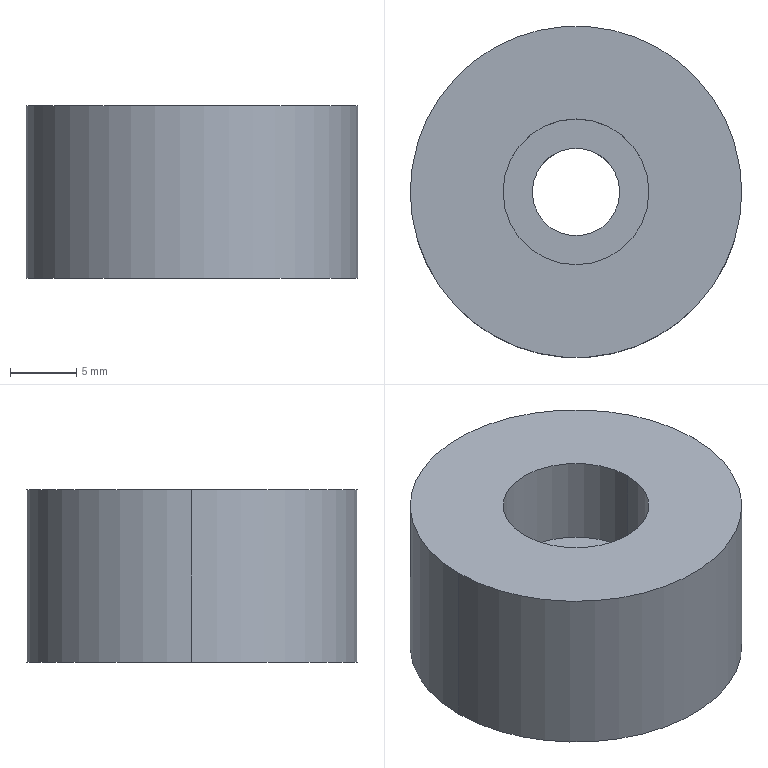Part | SolidWorks | features Extrusion 1, HoleWzd 1 | 1 solid | 9 faces | box 25 x 25 x 13 mm | volume 5523 mm3 | cylinder 6 | plane 3 | commonest cylinder face diameters 6.6 x2 11 x2 25 x2
STEP:
#1=CARTESIAN_POINT('',(-5.5,0.,6.2));
#2=VERTEX_POINT('',#1);
#3=CARTESIAN_POINT('',(5.5,0.,6.2));
#4=VERTEX_POINT('',#3);
#5=CARTESIAN_POINT('',(0.,0.,6.2));
#6=DIRECTION('',(0.,0.,1.));
#7=DIRECTION('',(1.,0.,0.));
#8=AXIS2_PLACEMENT_3D('',#5,#6,#7);
#9=CIRCLE('',#8,5.5);
#10=EDGE_CURVE('',#2,#4,#9,.T.);
#11=ORIENTED_EDGE('',*,*,#10,.F.);
#12=CARTESIAN_POINT('',(-5.5,0.,13.));
#13=VERTEX_POINT('',#12);
#14=CARTESIAN_POINT('',(-5.5,0.,13.));
#15=DIRECTION('',(0.,0.,1.));
#16=VECTOR('',#15,1000.);
#17=LINE('',#14,#16);
#18=EDGE_CURVE('',#2,#13,#17,.T.);
#19=ORIENTED_EDGE('',*,*,#18,.T.);
#20=CARTESIAN_POINT('',(5.5,0.,13.));
#21=VERTEX_POINT('',#20);
#22=CARTESIAN_POINT('',(0.,0.,13.));
#23=DIRECTION('',(0.,0.,1.));
#24=DIRECTION('',(1.,0.,0.));
#25=AXIS2_PLACEMENT_3D('',#22,#23,#24);
#26=CIRCLE('',#25,5.5);
#27=EDGE_CURVE('',#13,#21,#26,.T.);
#28=ORIENTED_EDGE('',*,*,#27,.T.);
#29=CARTESIAN_POINT('',(5.5,0.,13.));
#30=DIRECTION('',(0.,0.,1.));
#31=VECTOR('',#30,1000.);
#32=LINE('',#29,#31);
#33=EDGE_CURVE('',#4,#21,#32,.T.);
#34=ORIENTED_EDGE('',*,*,#33,.F.);
#35=EDGE_LOOP('',(#11,#19,#28,#34));
#36=FACE_OUTER_BOUND('',#35,.T.);
#37=CARTESIAN_POINT('',(0.,0.,13.));
#38=DIRECTION('',(0.,0.,1.));
#39=DIRECTION('',(1.,0.,0.));
#40=AXIS2_PLACEMENT_3D('',#37,#38,#39);
#41=CYLINDRICAL_SURFACE('',#40,5.5);
#42=ADVANCED_FACE('',(#36),#41,.F.);
#43=CARTESIAN_POINT('',(-3.3,0.,0.));
#44=VERTEX_POINT('',#43);
#45=CARTESIAN_POINT('',(3.3,0.,0.));
#46=VERTEX_POINT('',#45);
#47=CARTESIAN_POINT('',(0.,0.,0.));
#48=DIRECTION('',(0.,0.,1.));
#49=DIRECTION('',(1.,0.,0.));
#50=AXIS2_PLACEMENT_3D('',#47,#48,#49);
#51=CIRCLE('',#50,3.3);
#52=EDGE_CURVE('',#44,#46,#51,.T.);
#53=ORIENTED_EDGE('',*,*,#52,.F.);
#54=CARTESIAN_POINT('',(-3.3,0.,6.2));
#55=VERTEX_POINT('',#54);
#56=CARTESIAN_POINT('',(-3.3,0.,13.));
#57=DIRECTION('',(0.,0.,1.));
#58=VECTOR('',#57,1000.);
#59=LINE('',#56,#58);
#60=EDGE_CURVE('',#44,#55,#59,.T.);
#61=ORIENTED_EDGE('',*,*,#60,.T.);
#62=CARTESIAN_POINT('',(3.3,0.,6.2));
#63=VERTEX_POINT('',#62);
#64=CARTESIAN_POINT('',(0.,0.,6.2));
#65=DIRECTION('',(0.,0.,1.));
#66=DIRECTION('',(1.,0.,0.));
#67=AXIS2_PLACEMENT_3D('',#64,#65,#66);
#68=CIRCLE('',#67,3.3);
#69=EDGE_CURVE('',#55,#63,#68,.T.);
#70=ORIENTED_EDGE('',*,*,#69,.T.);
#71=CARTESIAN_POINT('',(3.3,0.,13.));
#72=DIRECTION('',(0.,0.,1.));
#73=VECTOR('',#72,1000.);
#74=LINE('',#71,#73);
#75=EDGE_CURVE('',#46,#63,#74,.T.);
#76=ORIENTED_EDGE('',*,*,#75,.F.);
#77=EDGE_LOOP('',(#53,#61,#70,#76));
#78=FACE_OUTER_BOUND('',#77,.T.);
#79=CARTESIAN_POINT('',(0.,0.,13.));
#80=DIRECTION('',(0.,0.,1.));
#81=DIRECTION('',(1.,0.,0.));
#82=AXIS2_PLACEMENT_3D('',#79,#80,#81);
#83=CYLINDRICAL_SURFACE('',#82,3.3);
#84=ADVANCED_FACE('',(#78),#83,.F.);
#85=CARTESIAN_POINT('',(12.5,0.,13.));
#86=VERTEX_POINT('',#85);
#87=CARTESIAN_POINT('',(-12.5,0.,13.));
#88=VERTEX_POINT('',#87);
#89=CARTESIAN_POINT('',(0.,0.,13.));
#90=DIRECTION('',(0.,0.,1.));
#91=DIRECTION('',(1.,0.,0.));
#92=AXIS2_PLACEMENT_3D('',#89,#90,#91);
#93=CIRCLE('',#92,12.5);
#94=EDGE_CURVE('',#86,#88,#93,.T.);
#95=ORIENTED_EDGE('',*,*,#94,.F.);
#96=CARTESIAN_POINT('',(12.5,0.,0.));
#97=VERTEX_POINT('',#96);
#98=CARTESIAN_POINT('',(12.5,0.,13.));
#99=DIRECTION('',(0.,0.,-1.));
#100=VECTOR('',#99,1000.);
#101=LINE('',#98,#100);
#102=EDGE_CURVE('',#86,#97,#101,.T.);
#103=ORIENTED_EDGE('',*,*,#102,.T.);
#104=CARTESIAN_POINT('',(-12.5,0.,0.));
#105=VERTEX_POINT('',#104);
#106=CARTESIAN_POINT('',(0.,0.,0.));
#107=DIRECTION('',(0.,0.,1.));
#108=DIRECTION('',(1.,0.,0.));
#109=AXIS2_PLACEMENT_3D('',#106,#107,#108);
#110=CIRCLE('',#109,12.5);
#111=EDGE_CURVE('',#97,#105,#110,.T.);
#112=ORIENTED_EDGE('',*,*,#111,.T.);
#113=CARTESIAN_POINT('',(-12.5,0.,13.));
#114=DIRECTION('',(0.,0.,-1.));
#115=VECTOR('',#114,1000.);
#116=LINE('',#113,#115);
#117=EDGE_CURVE('',#88,#105,#116,.T.);
#118=ORIENTED_EDGE('',*,*,#117,.F.);
#119=EDGE_LOOP('',(#95,#103,#112,#118));
#120=FACE_OUTER_BOUND('',#119,.T.);
#121=CARTESIAN_POINT('',(0.,0.,13.));
#122=DIRECTION('',(0.,0.,-1.));
#123=DIRECTION('',(-1.,0.,0.));
#124=AXIS2_PLACEMENT_3D('',#121,#122,#123);
#125=CYLINDRICAL_SURFACE('',#124,12.5);
#126=ADVANCED_FACE('',(#120),#125,.T.);
#127=ORIENTED_EDGE('',*,*,#102,.F.);
#128=CARTESIAN_POINT('',(0.,0.,13.));
#129=DIRECTION('',(0.,0.,1.));
#130=DIRECTION('',(1.,0.,0.));
#131=AXIS2_PLACEMENT_3D('',#128,#129,#130);
#132=CIRCLE('',#131,12.5);
#133=EDGE_CURVE('',#88,#86,#132,.T.);
#134=ORIENTED_EDGE('',*,*,#133,.F.);
#135=ORIENTED_EDGE('',*,*,#117,.T.);
#136=CARTESIAN_POINT('',(0.,0.,0.));
#137=DIRECTION('',(0.,0.,1.));
#138=DIRECTION('',(1.,0.,0.));
#139=AXIS2_PLACEMENT_3D('',#136,#137,#138);
#140=CIRCLE('',#139,12.5);
#141=EDGE_CURVE('',#105,#97,#140,.T.);
#142=ORIENTED_EDGE('',*,*,#141,.T.);
#143=EDGE_LOOP('',(#127,#134,#135,#142));
#144=FACE_OUTER_BOUND('',#143,.T.);
#145=CARTESIAN_POINT('',(0.,0.,13.));
#146=DIRECTION('',(0.,0.,-1.));
#147=DIRECTION('',(-1.,0.,0.));
#148=AXIS2_PLACEMENT_3D('',#145,#146,#147);
#149=CYLINDRICAL_SURFACE('',#148,12.5);
#150=ADVANCED_FACE('',(#144),#149,.T.);
#151=CARTESIAN_POINT('',(0.,0.,13.));
#152=DIRECTION('',(0.,0.,1.));
#153=DIRECTION('',(1.,0.,0.));
#154=AXIS2_PLACEMENT_3D('',#151,#152,#153);
#155=CIRCLE('',#154,5.5);
#156=EDGE_CURVE('',#21,#13,#155,.T.);
#157=ORIENTED_EDGE('',*,*,#156,.F.);
#158=ORIENTED_EDGE('',*,*,#27,.F.);
#159=EDGE_LOOP('',(#157,#158));
#160=FACE_BOUND('',#159,.T.);
#161=ORIENTED_EDGE('',*,*,#133,.T.);
#162=ORIENTED_EDGE('',*,*,#94,.T.);
#163=EDGE_LOOP('',(#161,#162));
#164=FACE_OUTER_BOUND('',#163,.T.);
#165=CARTESIAN_POINT('',(0.,0.,13.));
#166=DIRECTION('',(0.,0.,1.));
#167=DIRECTION('',(1.,0.,0.));
#168=AXIS2_PLACEMENT_3D('',#165,#166,#167);
#169=PLANE('',#168);
#170=ADVANCED_FACE('',(#160,#164),#169,.T.);
#171=CARTESIAN_POINT('',(0.,0.,0.));
#172=DIRECTION('',(0.,0.,1.));
#173=DIRECTION('',(1.,0.,0.));
#174=AXIS2_PLACEMENT_3D('',#171,#172,#173);
#175=CIRCLE('',#174,3.3);
#176=EDGE_CURVE('',#46,#44,#175,.T.);
#177=ORIENTED_EDGE('',*,*,#176,.T.);
#178=ORIENTED_EDGE('',*,*,#52,.T.);
#179=EDGE_LOOP('',(#177,#178));
#180=FACE_BOUND('',#179,.T.);
#181=ORIENTED_EDGE('',*,*,#141,.F.);
#182=ORIENTED_EDGE('',*,*,#111,.F.);
#183=EDGE_LOOP('',(#181,#182));
#184=FACE_OUTER_BOUND('',#183,.T.);
#185=CARTESIAN_POINT('',(0.,0.,0.));
#186=DIRECTION('',(0.,0.,1.));
#187=DIRECTION('',(1.,0.,0.));
#188=AXIS2_PLACEMENT_3D('',#185,#186,#187);
#189=PLANE('',#188);
#190=ADVANCED_FACE('',(#180,#184),#189,.F.);
#191=ORIENTED_EDGE('',*,*,#60,.F.);
#192=ORIENTED_EDGE('',*,*,#176,.F.);
#193=ORIENTED_EDGE('',*,*,#75,.T.);
#194=CARTESIAN_POINT('',(0.,0.,6.2));
#195=DIRECTION('',(0.,0.,1.));
#196=DIRECTION('',(1.,0.,0.));
#197=AXIS2_PLACEMENT_3D('',#194,#195,#196);
#198=CIRCLE('',#197,3.3);
#199=EDGE_CURVE('',#63,#55,#198,.T.);
#200=ORIENTED_EDGE('',*,*,#199,.T.);
#201=EDGE_LOOP('',(#191,#192,#193,#200));
#202=FACE_OUTER_BOUND('',#201,.T.);
#203=CARTESIAN_POINT('',(0.,0.,13.));
#204=DIRECTION('',(0.,0.,1.));
#205=DIRECTION('',(1.,0.,0.));
#206=AXIS2_PLACEMENT_3D('',#203,#204,#205);
#207=CYLINDRICAL_SURFACE('',#206,3.3);
#208=ADVANCED_FACE('',(#202),#207,.F.);
#209=ORIENTED_EDGE('',*,*,#199,.F.);
#210=ORIENTED_EDGE('',*,*,#69,.F.);
#211=EDGE_LOOP('',(#209,#210));
#212=FACE_BOUND('',#211,.T.);
#213=CARTESIAN_POINT('',(0.,0.,6.2));
#214=DIRECTION('',(0.,0.,1.));
#215=DIRECTION('',(1.,0.,0.));
#216=AXIS2_PLACEMENT_3D('',#213,#214,#215);
#217=CIRCLE('',#216,5.5);
#218=EDGE_CURVE('',#4,#2,#217,.T.);
#219=ORIENTED_EDGE('',*,*,#218,.T.);
#220=ORIENTED_EDGE('',*,*,#10,.T.);
#221=EDGE_LOOP('',(#219,#220));
#222=FACE_OUTER_BOUND('',#221,.T.);
#223=CARTESIAN_POINT('',(3.3,0.,6.2));
#224=DIRECTION('',(0.,0.,-1.));
#225=DIRECTION('',(-1.,0.,0.));
#226=AXIS2_PLACEMENT_3D('',#223,#224,#225);
#227=PLANE('',#226);
#228=ADVANCED_FACE('',(#212,#222),#227,.F.);
#229=ORIENTED_EDGE('',*,*,#18,.F.);
#230=ORIENTED_EDGE('',*,*,#218,.F.);
#231=ORIENTED_EDGE('',*,*,#33,.T.);
#232=ORIENTED_EDGE('',*,*,#156,.T.);
#233=EDGE_LOOP('',(#229,#230,#231,#232));
#234=FACE_OUTER_BOUND('',#233,.T.);
#235=CARTESIAN_POINT('',(0.,0.,13.));
#236=DIRECTION('',(0.,0.,1.));
#237=DIRECTION('',(1.,0.,0.));
#238=AXIS2_PLACEMENT_3D('',#235,#236,#237);
#239=CYLINDRICAL_SURFACE('',#238,5.5);
#240=ADVANCED_FACE('',(#234),#239,.F.);
#241=CLOSED_SHELL('',(#42,#84,#126,#150,#170,#190,#208,#228,#240));
#242=MANIFOLD_SOLID_BREP('',#241);
#243=CARTESIAN_POINT('',(0.,0.,0.));
#244=DIRECTION('',(0.,0.,1.));
#245=DIRECTION('',(1.,0.,0.));
#246=AXIS2_PLACEMENT_3D('',#243,#244,#245);
#247=(LENGTH_UNIT()NAMED_UNIT(*)SI_UNIT(.MILLI.,.METRE.));
#248=UNCERTAINTY_MEASURE_WITH_UNIT(LENGTH_MEASURE(0.00001),#247,'','');
#249=(NAMED_UNIT(*)PLANE_ANGLE_UNIT()SI_UNIT($,.RADIAN.));
#250=(NAMED_UNIT(*)SI_UNIT($,.STERADIAN.)SOLID_ANGLE_UNIT());
#251=(GEOMETRIC_REPRESENTATION_CONTEXT(3)GLOBAL_UNCERTAINTY_ASSIGNED_CONTEXT((#248))GLOBAL_UNIT_ASSIGNED_CONTEXT((#247,#249,#250))REPRESENTATION_CONTEXT('',''));
#252=ADVANCED_BREP_SHAPE_REPRESENTATION('',(#242,#246),#251);